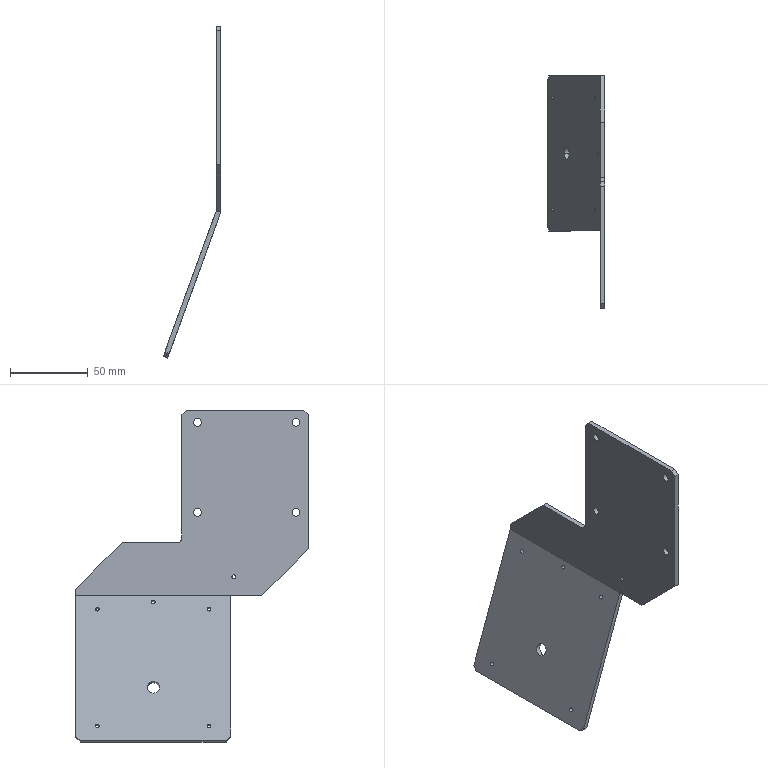Part | SolidWorks | features Chamfer 4, ICE 4, HoleWzd 3, 3DProfileFeature 1, Cut 1, Extrusion 1, Fillet 1, LPattern 1 | 1 solid | 49 faces | box 37.021 x 150 x 213.969 mm | volume 62969 mm3 | cylinder 23 | plane 18 | cone 8 | commonest cylinder face diameters 2.5 x12 5 x8 8 x2 6 x1